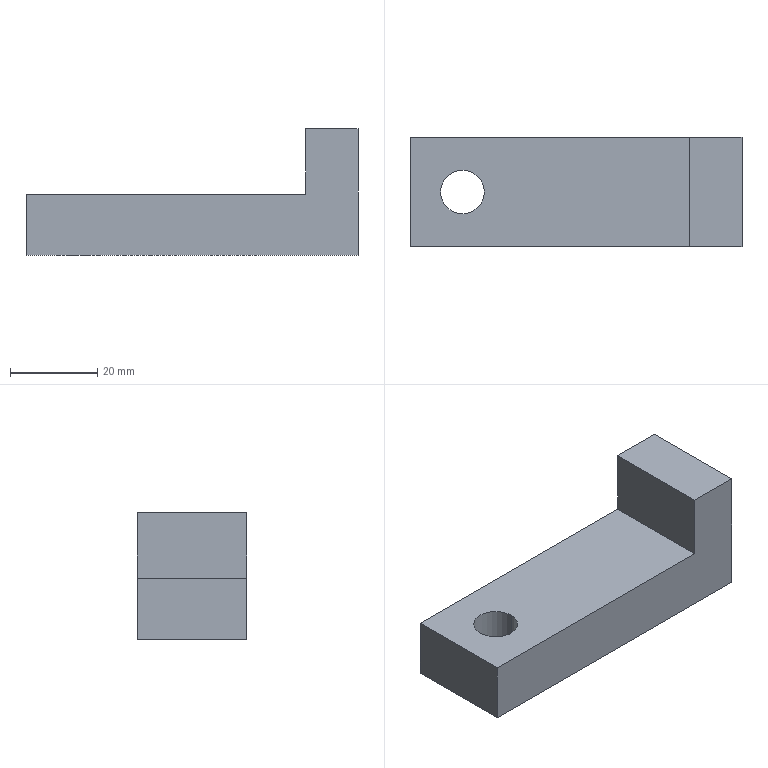Part | SolidWorks | features Extrusion 1, ICE 1 | 1 solid | 10 faces | box 76 x 25 x 29 mm | volume 30000 mm3 | plane 8 | cylinder 2 | commonest cylinder face diameters 10 x2
STEP:
#1=CARTESIAN_POINT('',(-31.,0.,7.));
#2=VERTEX_POINT('',#1);
#3=CARTESIAN_POINT('',(-21.,0.,7.));
#4=VERTEX_POINT('',#3);
#5=CARTESIAN_POINT('',(-26.,0.,7.));
#6=DIRECTION('',(0.,0.,1.));
#7=DIRECTION('',(1.,0.,0.));
#8=AXIS2_PLACEMENT_3D('',#5,#6,#7);
#9=CIRCLE('',#8,5.);
#10=EDGE_CURVE('',#2,#4,#9,.T.);
#11=ORIENTED_EDGE('',*,*,#10,.T.);
#12=CARTESIAN_POINT('',(-21.,0.,-7.));
#13=VERTEX_POINT('',#12);
#14=CARTESIAN_POINT('',(-21.,0.,7.));
#15=DIRECTION('',(0.,0.,-1.));
#16=VECTOR('',#15,1000.);
#17=LINE('',#14,#16);
#18=EDGE_CURVE('',#4,#13,#17,.T.);
#19=ORIENTED_EDGE('',*,*,#18,.T.);
#20=CARTESIAN_POINT('',(-31.,0.,-7.));
#21=VERTEX_POINT('',#20);
#22=CARTESIAN_POINT('',(-26.,0.,-7.));
#23=DIRECTION('',(0.,0.,1.));
#24=DIRECTION('',(1.,0.,0.));
#25=AXIS2_PLACEMENT_3D('',#22,#23,#24);
#26=CIRCLE('',#25,5.);
#27=EDGE_CURVE('',#21,#13,#26,.T.);
#28=ORIENTED_EDGE('',*,*,#27,.F.);
#29=CARTESIAN_POINT('',(-31.,0.,7.));
#30=DIRECTION('',(0.,0.,-1.));
#31=VECTOR('',#30,1000.);
#32=LINE('',#29,#31);
#33=EDGE_CURVE('',#2,#21,#32,.T.);
#34=ORIENTED_EDGE('',*,*,#33,.F.);
#35=EDGE_LOOP('',(#11,#19,#28,#34));
#36=FACE_OUTER_BOUND('',#35,.T.);
#37=CARTESIAN_POINT('',(-26.,0.,7.));
#38=DIRECTION('',(0.,0.,-1.));
#39=DIRECTION('',(-1.,0.,0.));
#40=AXIS2_PLACEMENT_3D('',#37,#38,#39);
#41=CYLINDRICAL_SURFACE('',#40,5.);
#42=ADVANCED_FACE('',(#36),#41,.F.);
#43=ORIENTED_EDGE('',*,*,#10,.F.);
#44=CARTESIAN_POINT('',(-26.,0.,7.));
#45=DIRECTION('',(0.,0.,1.));
#46=DIRECTION('',(1.,0.,0.));
#47=AXIS2_PLACEMENT_3D('',#44,#45,#46);
#48=CIRCLE('',#47,5.);
#49=EDGE_CURVE('',#4,#2,#48,.T.);
#50=ORIENTED_EDGE('',*,*,#49,.F.);
#51=EDGE_LOOP('',(#43,#50));
#52=FACE_BOUND('',#51,.T.);
#53=CARTESIAN_POINT('',(26.,12.5,7.));
#54=VERTEX_POINT('',#53);
#55=CARTESIAN_POINT('',(26.,-12.5,7.));
#56=VERTEX_POINT('',#55);
#57=CARTESIAN_POINT('',(26.,12.5,7.));
#58=DIRECTION('',(0.,-1.,0.));
#59=VECTOR('',#58,1000.);
#60=LINE('',#57,#59);
#61=EDGE_CURVE('',#54,#56,#60,.T.);
#62=ORIENTED_EDGE('',*,*,#61,.F.);
#63=CARTESIAN_POINT('',(-38.,12.5,7.));
#64=VERTEX_POINT('',#63);
#65=CARTESIAN_POINT('',(-38.,12.5,7.));
#66=DIRECTION('',(-1.,0.,0.));
#67=VECTOR('',#66,1000.);
#68=LINE('',#65,#67);
#69=EDGE_CURVE('',#54,#64,#68,.T.);
#70=ORIENTED_EDGE('',*,*,#69,.T.);
#71=CARTESIAN_POINT('',(-38.,-12.5,7.));
#72=VERTEX_POINT('',#71);
#73=CARTESIAN_POINT('',(-38.,-12.5,7.));
#74=DIRECTION('',(0.,-1.,0.));
#75=VECTOR('',#74,1000.);
#76=LINE('',#73,#75);
#77=EDGE_CURVE('',#64,#72,#76,.T.);
#78=ORIENTED_EDGE('',*,*,#77,.T.);
#79=CARTESIAN_POINT('',(-38.,-12.5,7.));
#80=DIRECTION('',(1.,0.,0.));
#81=VECTOR('',#80,1000.);
#82=LINE('',#79,#81);
#83=EDGE_CURVE('',#72,#56,#82,.T.);
#84=ORIENTED_EDGE('',*,*,#83,.T.);
#85=EDGE_LOOP('',(#62,#70,#78,#84));
#86=FACE_OUTER_BOUND('',#85,.T.);
#87=CARTESIAN_POINT('',(0.,0.,7.));
#88=DIRECTION('',(0.,0.,-1.));
#89=DIRECTION('',(-1.,0.,0.));
#90=AXIS2_PLACEMENT_3D('',#87,#88,#89);
#91=PLANE('',#90);
#92=ADVANCED_FACE('',(#52,#86),#91,.F.);
#93=CARTESIAN_POINT('',(38.,-12.5,-7.));
#94=VERTEX_POINT('',#93);
#95=CARTESIAN_POINT('',(38.,12.5,-7.));
#96=VERTEX_POINT('',#95);
#97=CARTESIAN_POINT('',(38.,-12.5,-7.));
#98=DIRECTION('',(0.,1.,0.));
#99=VECTOR('',#98,1000.);
#100=LINE('',#97,#99);
#101=EDGE_CURVE('',#94,#96,#100,.T.);
#102=ORIENTED_EDGE('',*,*,#101,.F.);
#103=CARTESIAN_POINT('',(-38.,-12.5,-7.));
#104=VERTEX_POINT('',#103);
#105=CARTESIAN_POINT('',(-38.,-12.5,-7.));
#106=DIRECTION('',(1.,0.,0.));
#107=VECTOR('',#106,1000.);
#108=LINE('',#105,#107);
#109=EDGE_CURVE('',#104,#94,#108,.T.);
#110=ORIENTED_EDGE('',*,*,#109,.F.);
#111=CARTESIAN_POINT('',(-38.,12.5,-7.));
#112=VERTEX_POINT('',#111);
#113=CARTESIAN_POINT('',(-38.,-12.5,-7.));
#114=DIRECTION('',(0.,-1.,0.));
#115=VECTOR('',#114,1000.);
#116=LINE('',#113,#115);
#117=EDGE_CURVE('',#112,#104,#116,.T.);
#118=ORIENTED_EDGE('',*,*,#117,.F.);
#119=CARTESIAN_POINT('',(-38.,12.5,-7.));
#120=DIRECTION('',(-1.,0.,0.));
#121=VECTOR('',#120,1000.);
#122=LINE('',#119,#121);
#123=EDGE_CURVE('',#96,#112,#122,.T.);
#124=ORIENTED_EDGE('',*,*,#123,.F.);
#125=EDGE_LOOP('',(#102,#110,#118,#124));
#126=FACE_OUTER_BOUND('',#125,.T.);
#127=ORIENTED_EDGE('',*,*,#27,.T.);
#128=CARTESIAN_POINT('',(-26.,0.,-7.));
#129=DIRECTION('',(0.,0.,1.));
#130=DIRECTION('',(1.,0.,0.));
#131=AXIS2_PLACEMENT_3D('',#128,#129,#130);
#132=CIRCLE('',#131,5.);
#133=EDGE_CURVE('',#13,#21,#132,.T.);
#134=ORIENTED_EDGE('',*,*,#133,.T.);
#135=EDGE_LOOP('',(#127,#134));
#136=FACE_BOUND('',#135,.T.);
#137=CARTESIAN_POINT('',(0.,0.,-7.));
#138=DIRECTION('',(0.,0.,-1.));
#139=DIRECTION('',(-1.,0.,0.));
#140=AXIS2_PLACEMENT_3D('',#137,#138,#139);
#141=PLANE('',#140);
#142=ADVANCED_FACE('',(#126,#136),#141,.T.);
#143=ORIENTED_EDGE('',*,*,#101,.T.);
#144=CARTESIAN_POINT('',(38.,12.5,22.));
#145=VERTEX_POINT('',#144);
#146=CARTESIAN_POINT('',(38.,12.5,7.));
#147=DIRECTION('',(0.,0.,-1.));
#148=VECTOR('',#147,1000.);
#149=LINE('',#146,#148);
#150=EDGE_CURVE('',#145,#96,#149,.T.);
#151=ORIENTED_EDGE('',*,*,#150,.F.);
#152=CARTESIAN_POINT('',(38.,-12.5,22.));
#153=VERTEX_POINT('',#152);
#154=CARTESIAN_POINT('',(38.,12.5,22.));
#155=DIRECTION('',(0.,1.,0.));
#156=VECTOR('',#155,1000.);
#157=LINE('',#154,#156);
#158=EDGE_CURVE('',#153,#145,#157,.T.);
#159=ORIENTED_EDGE('',*,*,#158,.F.);
#160=CARTESIAN_POINT('',(38.,-12.5,7.));
#161=DIRECTION('',(0.,0.,-1.));
#162=VECTOR('',#161,1000.);
#163=LINE('',#160,#162);
#164=EDGE_CURVE('',#153,#94,#163,.T.);
#165=ORIENTED_EDGE('',*,*,#164,.T.);
#166=EDGE_LOOP('',(#143,#151,#159,#165));
#167=FACE_OUTER_BOUND('',#166,.T.);
#168=CARTESIAN_POINT('',(38.,-12.5,7.));
#169=DIRECTION('',(-1.,0.,0.));
#170=DIRECTION('',(0.,-1.,0.));
#171=AXIS2_PLACEMENT_3D('',#168,#169,#170);
#172=PLANE('',#171);
#173=ADVANCED_FACE('',(#167),#172,.F.);
#174=ORIENTED_EDGE('',*,*,#123,.T.);
#175=CARTESIAN_POINT('',(-38.,12.5,7.));
#176=DIRECTION('',(0.,0.,-1.));
#177=VECTOR('',#176,1000.);
#178=LINE('',#175,#177);
#179=EDGE_CURVE('',#64,#112,#178,.T.);
#180=ORIENTED_EDGE('',*,*,#179,.F.);
#181=ORIENTED_EDGE('',*,*,#69,.F.);
#182=CARTESIAN_POINT('',(26.,12.5,22.));
#183=VERTEX_POINT('',#182);
#184=CARTESIAN_POINT('',(26.,12.5,22.));
#185=DIRECTION('',(0.,0.,-1.));
#186=VECTOR('',#185,1000.);
#187=LINE('',#184,#186);
#188=EDGE_CURVE('',#183,#54,#187,.T.);
#189=ORIENTED_EDGE('',*,*,#188,.F.);
#190=CARTESIAN_POINT('',(38.,12.5,22.));
#191=DIRECTION('',(-1.,0.,0.));
#192=VECTOR('',#191,1000.);
#193=LINE('',#190,#192);
#194=EDGE_CURVE('',#145,#183,#193,.T.);
#195=ORIENTED_EDGE('',*,*,#194,.F.);
#196=ORIENTED_EDGE('',*,*,#150,.T.);
#197=EDGE_LOOP('',(#174,#180,#181,#189,#195,#196));
#198=FACE_OUTER_BOUND('',#197,.T.);
#199=CARTESIAN_POINT('',(-38.,12.5,7.));
#200=DIRECTION('',(0.,-1.,0.));
#201=DIRECTION('',(0.,0.,-1.));
#202=AXIS2_PLACEMENT_3D('',#199,#200,#201);
#203=PLANE('',#202);
#204=ADVANCED_FACE('',(#198),#203,.F.);
#205=ORIENTED_EDGE('',*,*,#117,.T.);
#206=CARTESIAN_POINT('',(-38.,-12.5,7.));
#207=DIRECTION('',(0.,0.,-1.));
#208=VECTOR('',#207,1000.);
#209=LINE('',#206,#208);
#210=EDGE_CURVE('',#72,#104,#209,.T.);
#211=ORIENTED_EDGE('',*,*,#210,.F.);
#212=ORIENTED_EDGE('',*,*,#77,.F.);
#213=ORIENTED_EDGE('',*,*,#179,.T.);
#214=EDGE_LOOP('',(#205,#211,#212,#213));
#215=FACE_OUTER_BOUND('',#214,.T.);
#216=CARTESIAN_POINT('',(-38.,-12.5,7.));
#217=DIRECTION('',(1.,0.,0.));
#218=DIRECTION('',(0.,0.,-1.));
#219=AXIS2_PLACEMENT_3D('',#216,#217,#218);
#220=PLANE('',#219);
#221=ADVANCED_FACE('',(#215),#220,.F.);
#222=ORIENTED_EDGE('',*,*,#109,.T.);
#223=ORIENTED_EDGE('',*,*,#164,.F.);
#224=CARTESIAN_POINT('',(26.,-12.5,22.));
#225=VERTEX_POINT('',#224);
#226=CARTESIAN_POINT('',(38.,-12.5,22.));
#227=DIRECTION('',(1.,0.,0.));
#228=VECTOR('',#227,1000.);
#229=LINE('',#226,#228);
#230=EDGE_CURVE('',#225,#153,#229,.T.);
#231=ORIENTED_EDGE('',*,*,#230,.F.);
#232=CARTESIAN_POINT('',(26.,-12.5,22.));
#233=DIRECTION('',(0.,0.,-1.));
#234=VECTOR('',#233,1000.);
#235=LINE('',#232,#234);
#236=EDGE_CURVE('',#225,#56,#235,.T.);
#237=ORIENTED_EDGE('',*,*,#236,.T.);
#238=ORIENTED_EDGE('',*,*,#83,.F.);
#239=ORIENTED_EDGE('',*,*,#210,.T.);
#240=EDGE_LOOP('',(#222,#223,#231,#237,#238,#239));
#241=FACE_OUTER_BOUND('',#240,.T.);
#242=CARTESIAN_POINT('',(-38.,-12.5,7.));
#243=DIRECTION('',(0.,1.,0.));
#244=DIRECTION('',(0.,0.,1.));
#245=AXIS2_PLACEMENT_3D('',#242,#243,#244);
#246=PLANE('',#245);
#247=ADVANCED_FACE('',(#241),#246,.F.);
#248=ORIENTED_EDGE('',*,*,#18,.F.);
#249=ORIENTED_EDGE('',*,*,#49,.T.);
#250=ORIENTED_EDGE('',*,*,#33,.T.);
#251=ORIENTED_EDGE('',*,*,#133,.F.);
#252=EDGE_LOOP('',(#248,#249,#250,#251));
#253=FACE_OUTER_BOUND('',#252,.T.);
#254=CARTESIAN_POINT('',(-26.,0.,7.));
#255=DIRECTION('',(0.,0.,-1.));
#256=DIRECTION('',(-1.,0.,0.));
#257=AXIS2_PLACEMENT_3D('',#254,#255,#256);
#258=CYLINDRICAL_SURFACE('',#257,5.);
#259=ADVANCED_FACE('',(#253),#258,.F.);
#260=ORIENTED_EDGE('',*,*,#61,.T.);
#261=ORIENTED_EDGE('',*,*,#236,.F.);
#262=CARTESIAN_POINT('',(26.,12.5,22.));
#263=DIRECTION('',(0.,-1.,0.));
#264=VECTOR('',#263,1000.);
#265=LINE('',#262,#264);
#266=EDGE_CURVE('',#183,#225,#265,.T.);
#267=ORIENTED_EDGE('',*,*,#266,.F.);
#268=ORIENTED_EDGE('',*,*,#188,.T.);
#269=EDGE_LOOP('',(#260,#261,#267,#268));
#270=FACE_OUTER_BOUND('',#269,.T.);
#271=CARTESIAN_POINT('',(26.,12.5,22.));
#272=DIRECTION('',(1.,0.,0.));
#273=DIRECTION('',(0.,1.,0.));
#274=AXIS2_PLACEMENT_3D('',#271,#272,#273);
#275=PLANE('',#274);
#276=ADVANCED_FACE('',(#270),#275,.F.);
#277=ORIENTED_EDGE('',*,*,#158,.T.);
#278=ORIENTED_EDGE('',*,*,#194,.T.);
#279=ORIENTED_EDGE('',*,*,#266,.T.);
#280=ORIENTED_EDGE('',*,*,#230,.T.);
#281=EDGE_LOOP('',(#277,#278,#279,#280));
#282=FACE_OUTER_BOUND('',#281,.T.);
#283=CARTESIAN_POINT('',(0.,0.,22.));
#284=DIRECTION('',(0.,0.,-1.));
#285=DIRECTION('',(-1.,0.,0.));
#286=AXIS2_PLACEMENT_3D('',#283,#284,#285);
#287=PLANE('',#286);
#288=ADVANCED_FACE('',(#282),#287,.F.);
#289=CLOSED_SHELL('',(#42,#92,#142,#173,#204,#221,#247,#259,#276,#288));
#290=MANIFOLD_SOLID_BREP('',#289);
#291=CARTESIAN_POINT('',(0.,0.,0.));
#292=DIRECTION('',(0.,0.,1.));
#293=DIRECTION('',(1.,0.,0.));
#294=AXIS2_PLACEMENT_3D('',#291,#292,#293);
#295=(LENGTH_UNIT()NAMED_UNIT(*)SI_UNIT(.MILLI.,.METRE.));
#296=UNCERTAINTY_MEASURE_WITH_UNIT(LENGTH_MEASURE(0.00001),#295,'','');
#297=(NAMED_UNIT(*)PLANE_ANGLE_UNIT()SI_UNIT($,.RADIAN.));
#298=(NAMED_UNIT(*)SI_UNIT($,.STERADIAN.)SOLID_ANGLE_UNIT());
#299=(GEOMETRIC_REPRESENTATION_CONTEXT(3)GLOBAL_UNCERTAINTY_ASSIGNED_CONTEXT((#296))GLOBAL_UNIT_ASSIGNED_CONTEXT((#295,#297,#298))REPRESENTATION_CONTEXT('',''));
#300=ADVANCED_BREP_SHAPE_REPRESENTATION('',(#290,#294),#299);